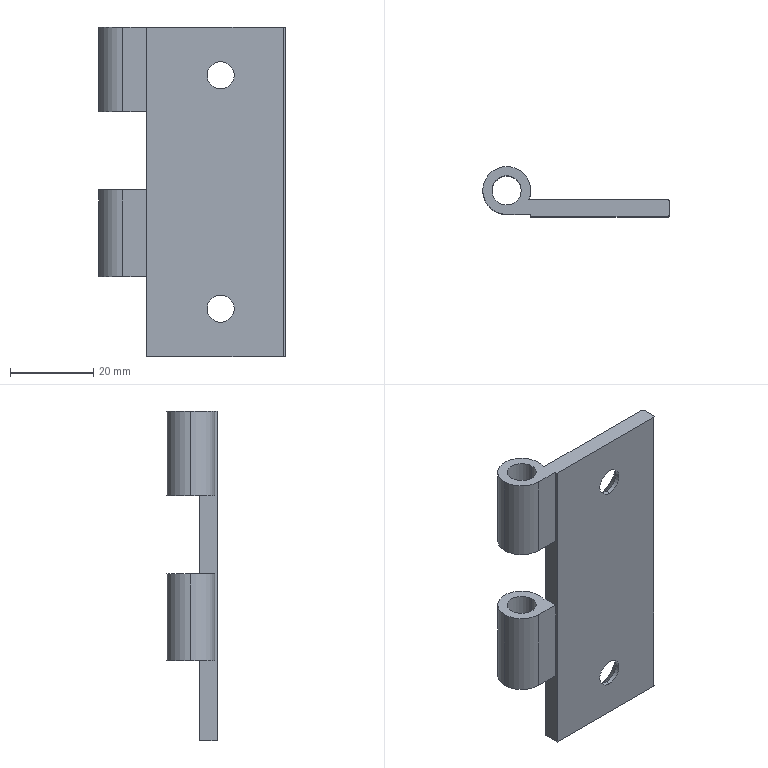Part | SolidWorks | features BaseBody 1 | 1 solid | 31 faces | box 44.75 x 12.05 x 79 mm | volume 13207 mm3 | cylinder 16 | plane 11 | cone 4 | commonest cylinder face diameters 11.5 x6 6.5 x4 7 x4 1 x2
STEP:
#1=CARTESIAN_POINT('',(23.5,0.,-24.75));
#2=VERTEX_POINT('',#1);
#3=CARTESIAN_POINT('',(23.5,0.,-31.25));
#4=VERTEX_POINT('',#3);
#5=CARTESIAN_POINT('',(23.5,0.,-28.));
#6=DIRECTION('',(0.,-1.,0.));
#7=DIRECTION('',(0.,0.,1.));
#8=AXIS2_PLACEMENT_3D('',#5,#6,#7);
#9=CIRCLE('',#8,3.25);
#10=EDGE_CURVE('',#2,#4,#9,.T.);
#11=ORIENTED_EDGE('',*,*,#10,.T.);
#12=CARTESIAN_POINT('',(23.5,1.1,-31.25));
#13=VERTEX_POINT('',#12);
#14=CARTESIAN_POINT('',(23.5,0.,-31.25));
#15=DIRECTION('',(0.,1.,0.));
#16=VECTOR('',#15,1000.);
#17=LINE('',#14,#16);
#18=EDGE_CURVE('',#4,#13,#17,.T.);
#19=ORIENTED_EDGE('',*,*,#18,.T.);
#20=CARTESIAN_POINT('',(23.5,1.1,-24.75));
#21=VERTEX_POINT('',#20);
#22=CARTESIAN_POINT('',(23.5,1.1,-28.));
#23=DIRECTION('',(0.,-1.,0.));
#24=DIRECTION('',(0.,0.,1.));
#25=AXIS2_PLACEMENT_3D('',#22,#23,#24);
#26=CIRCLE('',#25,3.25);
#27=EDGE_CURVE('',#21,#13,#26,.T.);
#28=ORIENTED_EDGE('',*,*,#27,.F.);
#29=CARTESIAN_POINT('',(23.5,0.,-24.75));
#30=DIRECTION('',(0.,1.,0.));
#31=VECTOR('',#30,1000.);
#32=LINE('',#29,#31);
#33=EDGE_CURVE('',#2,#21,#32,.T.);
#34=ORIENTED_EDGE('',*,*,#33,.F.);
#35=EDGE_LOOP('',(#11,#19,#28,#34));
#36=FACE_OUTER_BOUND('',#35,.T.);
#37=CARTESIAN_POINT('',(23.5,0.,-28.));
#38=DIRECTION('',(0.,1.,0.));
#39=DIRECTION('',(0.,0.,1.));
#40=AXIS2_PLACEMENT_3D('',#37,#38,#39);
#41=CYLINDRICAL_SURFACE('',#40,3.25);
#42=ADVANCED_FACE('',(#36),#41,.F.);
#43=CARTESIAN_POINT('',(23.5,0.,31.25));
#44=VERTEX_POINT('',#43);
#45=CARTESIAN_POINT('',(23.5,0.,24.75));
#46=VERTEX_POINT('',#45);
#47=CARTESIAN_POINT('',(23.5,0.,28.));
#48=DIRECTION('',(0.,-1.,0.));
#49=DIRECTION('',(0.,0.,1.));
#50=AXIS2_PLACEMENT_3D('',#47,#48,#49);
#51=CIRCLE('',#50,3.25);
#52=EDGE_CURVE('',#44,#46,#51,.T.);
#53=ORIENTED_EDGE('',*,*,#52,.T.);
#54=CARTESIAN_POINT('',(23.5,1.1,24.75));
#55=VERTEX_POINT('',#54);
#56=CARTESIAN_POINT('',(23.5,0.,24.75));
#57=DIRECTION('',(0.,1.,0.));
#58=VECTOR('',#57,1000.);
#59=LINE('',#56,#58);
#60=EDGE_CURVE('',#46,#55,#59,.T.);
#61=ORIENTED_EDGE('',*,*,#60,.T.);
#62=CARTESIAN_POINT('',(23.5,1.1,31.25));
#63=VERTEX_POINT('',#62);
#64=CARTESIAN_POINT('',(23.5,1.1,28.));
#65=DIRECTION('',(0.,-1.,0.));
#66=DIRECTION('',(0.,0.,1.));
#67=AXIS2_PLACEMENT_3D('',#64,#65,#66);
#68=CIRCLE('',#67,3.25);
#69=EDGE_CURVE('',#63,#55,#68,.T.);
#70=ORIENTED_EDGE('',*,*,#69,.F.);
#71=CARTESIAN_POINT('',(23.5,0.,31.25));
#72=DIRECTION('',(0.,1.,0.));
#73=VECTOR('',#72,1000.);
#74=LINE('',#71,#73);
#75=EDGE_CURVE('',#44,#63,#74,.T.);
#76=ORIENTED_EDGE('',*,*,#75,.F.);
#77=EDGE_LOOP('',(#53,#61,#70,#76));
#78=FACE_OUTER_BOUND('',#77,.T.);
#79=CARTESIAN_POINT('',(23.5,0.,28.));
#80=DIRECTION('',(0.,1.,0.));
#81=DIRECTION('',(0.,0.,1.));
#82=AXIS2_PLACEMENT_3D('',#79,#80,#81);
#83=CYLINDRICAL_SURFACE('',#82,3.25);
#84=ADVANCED_FACE('',(#78),#83,.F.);
#85=CARTESIAN_POINT('',(5.75,6.3,19.3));
#86=VERTEX_POINT('',#85);
#87=CARTESIAN_POINT('',(-5.75,6.3,19.3));
#88=VERTEX_POINT('',#87);
#89=CARTESIAN_POINT('',(0.,6.3,19.3));
#90=DIRECTION('',(0.,0.,1.));
#91=DIRECTION('',(1.,0.,0.));
#92=AXIS2_PLACEMENT_3D('',#89,#90,#91);
#93=CIRCLE('',#92,5.75);
#94=EDGE_CURVE('',#86,#88,#93,.T.);
#95=ORIENTED_EDGE('',*,*,#94,.T.);
#96=CARTESIAN_POINT('',(-5.75,6.3,39.5));
#97=VERTEX_POINT('',#96);
#98=CARTESIAN_POINT('',(-5.75,6.3,39.5));
#99=DIRECTION('',(0.,0.,1.));
#100=VECTOR('',#99,1000.);
#101=LINE('',#98,#100);
#102=EDGE_CURVE('',#88,#97,#101,.T.);
#103=ORIENTED_EDGE('',*,*,#102,.T.);
#104=CARTESIAN_POINT('',(5.75,6.3,39.5));
#105=VERTEX_POINT('',#104);
#106=CARTESIAN_POINT('',(0.,6.3,39.5));
#107=DIRECTION('',(0.,0.,1.));
#108=DIRECTION('',(1.,0.,0.));
#109=AXIS2_PLACEMENT_3D('',#106,#107,#108);
#110=CIRCLE('',#109,5.75);
#111=EDGE_CURVE('',#105,#97,#110,.T.);
#112=ORIENTED_EDGE('',*,*,#111,.F.);
#113=CARTESIAN_POINT('',(5.75,6.3,39.5));
#114=DIRECTION('',(0.,0.,1.));
#115=VECTOR('',#114,1000.);
#116=LINE('',#113,#115);
#117=EDGE_CURVE('',#86,#105,#116,.T.);
#118=ORIENTED_EDGE('',*,*,#117,.F.);
#119=EDGE_LOOP('',(#95,#103,#112,#118));
#120=FACE_OUTER_BOUND('',#119,.T.);
#121=CARTESIAN_POINT('',(0.,6.3,39.5));
#122=DIRECTION('',(0.,0.,1.));
#123=DIRECTION('',(1.,0.,0.));
#124=AXIS2_PLACEMENT_3D('',#121,#122,#123);
#125=CYLINDRICAL_SURFACE('',#124,5.75);
#126=ADVANCED_FACE('',(#120),#125,.T.);
#127=CARTESIAN_POINT('',(5.312,4.1,19.3));
#128=VERTEX_POINT('',#127);
#129=CARTESIAN_POINT('',(0.,6.3,19.3));
#130=DIRECTION('',(0.,0.,1.));
#131=DIRECTION('',(1.,0.,0.));
#132=AXIS2_PLACEMENT_3D('',#129,#130,#131);
#133=CIRCLE('',#132,5.75);
#134=EDGE_CURVE('',#128,#86,#133,.T.);
#135=ORIENTED_EDGE('',*,*,#134,.T.);
#136=ORIENTED_EDGE('',*,*,#117,.T.);
#137=CARTESIAN_POINT('',(5.312,4.1,39.5));
#138=VERTEX_POINT('',#137);
#139=CARTESIAN_POINT('',(0.,6.3,39.5));
#140=DIRECTION('',(0.,0.,1.));
#141=DIRECTION('',(1.,0.,0.));
#142=AXIS2_PLACEMENT_3D('',#139,#140,#141);
#143=CIRCLE('',#142,5.75);
#144=EDGE_CURVE('',#138,#105,#143,.T.);
#145=ORIENTED_EDGE('',*,*,#144,.F.);
#146=CARTESIAN_POINT('',(5.312,4.1,39.5));
#147=DIRECTION('',(0.,0.,-1.));
#148=VECTOR('',#147,1000.);
#149=LINE('',#146,#148);
#150=EDGE_CURVE('',#138,#128,#149,.T.);
#151=ORIENTED_EDGE('',*,*,#150,.T.);
#152=EDGE_LOOP('',(#135,#136,#145,#151));
#153=FACE_OUTER_BOUND('',#152,.T.);
#154=CARTESIAN_POINT('',(0.,6.3,39.5));
#155=DIRECTION('',(0.,0.,1.));
#156=DIRECTION('',(1.,0.,0.));
#157=AXIS2_PLACEMENT_3D('',#154,#155,#156);
#158=CYLINDRICAL_SURFACE('',#157,5.75);
#159=ADVANCED_FACE('',(#153),#158,.T.);
#160=CARTESIAN_POINT('',(-3.5,6.3,19.3));
#161=VERTEX_POINT('',#160);
#162=CARTESIAN_POINT('',(3.5,6.3,19.3));
#163=VERTEX_POINT('',#162);
#164=CARTESIAN_POINT('',(0.,6.3,19.3));
#165=DIRECTION('',(0.,0.,1.));
#166=DIRECTION('',(1.,0.,0.));
#167=AXIS2_PLACEMENT_3D('',#164,#165,#166);
#168=CIRCLE('',#167,3.5);
#169=EDGE_CURVE('',#161,#163,#168,.T.);
#170=ORIENTED_EDGE('',*,*,#169,.F.);
#171=CARTESIAN_POINT('',(-3.5,6.3,39.5));
#172=VERTEX_POINT('',#171);
#173=CARTESIAN_POINT('',(-3.5,6.3,39.5));
#174=DIRECTION('',(0.,0.,1.));
#175=VECTOR('',#174,1000.);
#176=LINE('',#173,#175);
#177=EDGE_CURVE('',#161,#172,#176,.T.);
#178=ORIENTED_EDGE('',*,*,#177,.T.);
#179=CARTESIAN_POINT('',(3.5,6.3,39.5));
#180=VERTEX_POINT('',#179);
#181=CARTESIAN_POINT('',(0.,6.3,39.5));
#182=DIRECTION('',(0.,0.,-1.));
#183=DIRECTION('',(1.,0.,0.));
#184=AXIS2_PLACEMENT_3D('',#181,#182,#183);
#185=CIRCLE('',#184,3.5);
#186=EDGE_CURVE('',#180,#172,#185,.T.);
#187=ORIENTED_EDGE('',*,*,#186,.F.);
#188=CARTESIAN_POINT('',(3.5,6.3,39.5));
#189=DIRECTION('',(0.,0.,1.));
#190=VECTOR('',#189,1000.);
#191=LINE('',#188,#190);
#192=EDGE_CURVE('',#163,#180,#191,.T.);
#193=ORIENTED_EDGE('',*,*,#192,.F.);
#194=EDGE_LOOP('',(#170,#178,#187,#193));
#195=FACE_OUTER_BOUND('',#194,.T.);
#196=CARTESIAN_POINT('',(0.,6.3,39.5));
#197=DIRECTION('',(0.,0.,1.));
#198=DIRECTION('',(1.,0.,0.));
#199=AXIS2_PLACEMENT_3D('',#196,#197,#198);
#200=CYLINDRICAL_SURFACE('',#199,3.5);
#201=ADVANCED_FACE('',(#195),#200,.F.);
#202=ORIENTED_EDGE('',*,*,#27,.T.);
#203=CARTESIAN_POINT('',(23.5,4.1,-34.25));
#204=VERTEX_POINT('',#203);
#205=CARTESIAN_POINT('',(23.5,4.1,-34.25));
#206=DIRECTION('',(0.,0.7071,-0.7071));
#207=VECTOR('',#206,1000.);
#208=LINE('',#205,#207);
#209=EDGE_CURVE('',#13,#204,#208,.T.);
#210=ORIENTED_EDGE('',*,*,#209,.T.);
#211=CARTESIAN_POINT('',(23.5,4.1,-21.75));
#212=VERTEX_POINT('',#211);
#213=CARTESIAN_POINT('',(23.5,4.1,-28.));
#214=DIRECTION('',(0.,1.,0.));
#215=DIRECTION('',(0.,0.,1.));
#216=AXIS2_PLACEMENT_3D('',#213,#214,#215);
#217=CIRCLE('',#216,6.25);
#218=EDGE_CURVE('',#204,#212,#217,.T.);
#219=ORIENTED_EDGE('',*,*,#218,.T.);
#220=CARTESIAN_POINT('',(23.5,4.1,-21.75));
#221=DIRECTION('',(0.,0.7071,0.7071));
#222=VECTOR('',#221,1000.);
#223=LINE('',#220,#222);
#224=EDGE_CURVE('',#21,#212,#223,.T.);
#225=ORIENTED_EDGE('',*,*,#224,.F.);
#226=EDGE_LOOP('',(#202,#210,#219,#225));
#227=FACE_OUTER_BOUND('',#226,.T.);
#228=CARTESIAN_POINT('',(23.5,4.1,-28.));
#229=DIRECTION('',(0.,1.,0.));
#230=DIRECTION('',(0.,0.,1.));
#231=AXIS2_PLACEMENT_3D('',#228,#229,#230);
#232=CONICAL_SURFACE('',#231,6.25,0.7854);
#233=ADVANCED_FACE('',(#227),#232,.F.);
#234=ORIENTED_EDGE('',*,*,#69,.T.);
#235=CARTESIAN_POINT('',(23.5,4.1,21.75));
#236=VERTEX_POINT('',#235);
#237=CARTESIAN_POINT('',(23.5,4.1,21.75));
#238=DIRECTION('',(0.,0.7071,-0.7071));
#239=VECTOR('',#238,1000.);
#240=LINE('',#237,#239);
#241=EDGE_CURVE('',#55,#236,#240,.T.);
#242=ORIENTED_EDGE('',*,*,#241,.T.);
#243=CARTESIAN_POINT('',(23.5,4.1,34.25));
#244=VERTEX_POINT('',#243);
#245=CARTESIAN_POINT('',(23.5,4.1,28.));
#246=DIRECTION('',(0.,1.,0.));
#247=DIRECTION('',(0.,0.,1.));
#248=AXIS2_PLACEMENT_3D('',#245,#246,#247);
#249=CIRCLE('',#248,6.25);
#250=EDGE_CURVE('',#236,#244,#249,.T.);
#251=ORIENTED_EDGE('',*,*,#250,.T.);
#252=CARTESIAN_POINT('',(23.5,4.1,34.25));
#253=DIRECTION('',(0.,0.7071,0.7071));
#254=VECTOR('',#253,1000.);
#255=LINE('',#252,#254);
#256=EDGE_CURVE('',#63,#244,#255,.T.);
#257=ORIENTED_EDGE('',*,*,#256,.F.);
#258=EDGE_LOOP('',(#234,#242,#251,#257));
#259=FACE_OUTER_BOUND('',#258,.T.);
#260=CARTESIAN_POINT('',(23.5,4.1,28.));
#261=DIRECTION('',(0.,1.,0.));
#262=DIRECTION('',(0.,0.,1.));
#263=AXIS2_PLACEMENT_3D('',#260,#261,#262);
#264=CONICAL_SURFACE('',#263,6.25,0.7854);
#265=ADVANCED_FACE('',(#259),#264,.F.);
#266=CARTESIAN_POINT('',(-5.75,6.3,-20.3));
#267=VERTEX_POINT('',#266);
#268=CARTESIAN_POINT('',(5.75,6.3,-20.3));
#269=VERTEX_POINT('',#268);
#270=CARTESIAN_POINT('',(0.,6.3,-20.3));
#271=DIRECTION('',(0.,0.,-1.));
#272=DIRECTION('',(1.,0.,0.));
#273=AXIS2_PLACEMENT_3D('',#270,#271,#272);
#274=CIRCLE('',#273,5.75);
#275=EDGE_CURVE('',#267,#269,#274,.T.);
#276=ORIENTED_EDGE('',*,*,#275,.F.);
#277=CARTESIAN_POINT('',(-5.75,6.3,0.5));
#278=VERTEX_POINT('',#277);
#279=CARTESIAN_POINT('',(-5.75,6.3,39.5));
#280=DIRECTION('',(0.,0.,1.));
#281=VECTOR('',#280,1000.);
#282=LINE('',#279,#281);
#283=EDGE_CURVE('',#267,#278,#282,.T.);
#284=ORIENTED_EDGE('',*,*,#283,.T.);
#285=CARTESIAN_POINT('',(5.75,6.3,0.5));
#286=VERTEX_POINT('',#285);
#287=CARTESIAN_POINT('',(0.,6.3,0.5));
#288=DIRECTION('',(0.,0.,1.));
#289=DIRECTION('',(1.,0.,0.));
#290=AXIS2_PLACEMENT_3D('',#287,#288,#289);
#291=CIRCLE('',#290,5.75);
#292=EDGE_CURVE('',#286,#278,#291,.T.);
#293=ORIENTED_EDGE('',*,*,#292,.F.);
#294=CARTESIAN_POINT('',(5.75,6.3,39.5));
#295=DIRECTION('',(0.,0.,1.));
#296=VECTOR('',#295,1000.);
#297=LINE('',#294,#296);
#298=EDGE_CURVE('',#269,#286,#297,.T.);
#299=ORIENTED_EDGE('',*,*,#298,.F.);
#300=EDGE_LOOP('',(#276,#284,#293,#299));
#301=FACE_OUTER_BOUND('',#300,.T.);
#302=CARTESIAN_POINT('',(0.,6.3,39.5));
#303=DIRECTION('',(0.,0.,1.));
#304=DIRECTION('',(1.,0.,0.));
#305=AXIS2_PLACEMENT_3D('',#302,#303,#304);
#306=CYLINDRICAL_SURFACE('',#305,5.75);
#307=ADVANCED_FACE('',(#301),#306,.T.);
#308=CARTESIAN_POINT('',(5.312,4.1,-20.3));
#309=VERTEX_POINT('',#308);
#310=CARTESIAN_POINT('',(0.,6.3,-20.3));
#311=DIRECTION('',(0.,0.,-1.));
#312=DIRECTION('',(1.,0.,0.));
#313=AXIS2_PLACEMENT_3D('',#310,#311,#312);
#314=CIRCLE('',#313,5.75);
#315=EDGE_CURVE('',#269,#309,#314,.T.);
#316=ORIENTED_EDGE('',*,*,#315,.F.);
#317=ORIENTED_EDGE('',*,*,#298,.T.);
#318=CARTESIAN_POINT('',(5.312,4.1,0.5));
#319=VERTEX_POINT('',#318);
#320=CARTESIAN_POINT('',(0.,6.3,0.5));
#321=DIRECTION('',(0.,0.,1.));
#322=DIRECTION('',(1.,0.,0.));
#323=AXIS2_PLACEMENT_3D('',#320,#321,#322);
#324=CIRCLE('',#323,5.75);
#325=EDGE_CURVE('',#319,#286,#324,.T.);
#326=ORIENTED_EDGE('',*,*,#325,.F.);
#327=CARTESIAN_POINT('',(5.312,4.1,39.5));
#328=DIRECTION('',(0.,0.,-1.));
#329=VECTOR('',#328,1000.);
#330=LINE('',#327,#329);
#331=EDGE_CURVE('',#319,#309,#330,.T.);
#332=ORIENTED_EDGE('',*,*,#331,.T.);
#333=EDGE_LOOP('',(#316,#317,#326,#332));
#334=FACE_OUTER_BOUND('',#333,.T.);
#335=CARTESIAN_POINT('',(0.,6.3,39.5));
#336=DIRECTION('',(0.,0.,1.));
#337=DIRECTION('',(1.,0.,0.));
#338=AXIS2_PLACEMENT_3D('',#335,#336,#337);
#339=CYLINDRICAL_SURFACE('',#338,5.75);
#340=ADVANCED_FACE('',(#334),#339,.T.);
#341=CARTESIAN_POINT('',(-3.5,6.3,-20.3));
#342=VERTEX_POINT('',#341);
#343=CARTESIAN_POINT('',(3.5,6.3,-20.3));
#344=VERTEX_POINT('',#343);
#345=CARTESIAN_POINT('',(0.,6.3,-20.3));
#346=DIRECTION('',(0.,0.,1.));
#347=DIRECTION('',(1.,0.,0.));
#348=AXIS2_PLACEMENT_3D('',#345,#346,#347);
#349=CIRCLE('',#348,3.5);
#350=EDGE_CURVE('',#342,#344,#349,.T.);
#351=ORIENTED_EDGE('',*,*,#350,.F.);
#352=CARTESIAN_POINT('',(-3.5,6.3,0.5));
#353=VERTEX_POINT('',#352);
#354=CARTESIAN_POINT('',(-3.5,6.3,39.5));
#355=DIRECTION('',(0.,0.,1.));
#356=VECTOR('',#355,1000.);
#357=LINE('',#354,#356);
#358=EDGE_CURVE('',#342,#353,#357,.T.);
#359=ORIENTED_EDGE('',*,*,#358,.T.);
#360=CARTESIAN_POINT('',(3.5,6.3,0.5));
#361=VERTEX_POINT('',#360);
#362=CARTESIAN_POINT('',(0.,6.3,0.5));
#363=DIRECTION('',(0.,0.,-1.));
#364=DIRECTION('',(1.,0.,0.));
#365=AXIS2_PLACEMENT_3D('',#362,#363,#364);
#366=CIRCLE('',#365,3.5);
#367=EDGE_CURVE('',#361,#353,#366,.T.);
#368=ORIENTED_EDGE('',*,*,#367,.F.);
#369=CARTESIAN_POINT('',(3.5,6.3,39.5));
#370=DIRECTION('',(0.,0.,1.));
#371=VECTOR('',#370,1000.);
#372=LINE('',#369,#371);
#373=EDGE_CURVE('',#344,#361,#372,.T.);
#374=ORIENTED_EDGE('',*,*,#373,.F.);
#375=EDGE_LOOP('',(#351,#359,#368,#374));
#376=FACE_OUTER_BOUND('',#375,.T.);
#377=CARTESIAN_POINT('',(0.,6.3,39.5));
#378=DIRECTION('',(0.,0.,1.));
#379=DIRECTION('',(1.,0.,0.));
#380=AXIS2_PLACEMENT_3D('',#377,#378,#379);
#381=CYLINDRICAL_SURFACE('',#380,3.5);
#382=ADVANCED_FACE('',(#376),#381,.F.);
#383=CARTESIAN_POINT('',(38.5,0.,39.5));
#384=VERTEX_POINT('',#383);
#385=CARTESIAN_POINT('',(38.5,0.,-39.5));
#386=VERTEX_POINT('',#385);
#387=CARTESIAN_POINT('',(38.5,0.,39.5));
#388=DIRECTION('',(0.,0.,-1.));
#389=VECTOR('',#388,1000.);
#390=LINE('',#387,#389);
#391=EDGE_CURVE('',#384,#386,#390,.T.);
#392=ORIENTED_EDGE('',*,*,#391,.F.);
#393=CARTESIAN_POINT('',(5.75,0.,39.5));
#394=VERTEX_POINT('',#393);
#395=CARTESIAN_POINT('',(5.75,0.,39.5));
#396=DIRECTION('',(1.,0.,0.));
#397=VECTOR('',#396,1000.);
#398=LINE('',#395,#397);
#399=EDGE_CURVE('',#394,#384,#398,.T.);
#400=ORIENTED_EDGE('',*,*,#399,.F.);
#401=CARTESIAN_POINT('',(5.75,0.,-39.5));
#402=VERTEX_POINT('',#401);
#403=CARTESIAN_POINT('',(5.75,0.,39.5));
#404=DIRECTION('',(0.,0.,1.));
#405=VECTOR('',#404,1000.);
#406=LINE('',#403,#405);
#407=EDGE_CURVE('',#402,#394,#406,.T.);
#408=ORIENTED_EDGE('',*,*,#407,.F.);
#409=CARTESIAN_POINT('',(5.75,0.,-39.5));
#410=DIRECTION('',(-1.,0.,0.));
#411=VECTOR('',#410,1000.);
#412=LINE('',#409,#411);
#413=EDGE_CURVE('',#386,#402,#412,.T.);
#414=ORIENTED_EDGE('',*,*,#413,.F.);
#415=EDGE_LOOP('',(#392,#400,#408,#414));
#416=FACE_OUTER_BOUND('',#415,.T.);
#417=ORIENTED_EDGE('',*,*,#10,.F.);
#418=CARTESIAN_POINT('',(23.5,0.,-28.));
#419=DIRECTION('',(0.,-1.,0.));
#420=DIRECTION('',(0.,0.,1.));
#421=AXIS2_PLACEMENT_3D('',#418,#419,#420);
#422=CIRCLE('',#421,3.25);
#423=EDGE_CURVE('',#4,#2,#422,.T.);
#424=ORIENTED_EDGE('',*,*,#423,.F.);
#425=EDGE_LOOP('',(#417,#424));
#426=FACE_BOUND('',#425,.T.);
#427=ORIENTED_EDGE('',*,*,#52,.F.);
#428=CARTESIAN_POINT('',(23.5,0.,28.));
#429=DIRECTION('',(0.,-1.,0.));
#430=DIRECTION('',(0.,0.,1.));
#431=AXIS2_PLACEMENT_3D('',#428,#429,#430);
#432=CIRCLE('',#431,3.25);
#433=EDGE_CURVE('',#46,#44,#432,.T.);
#434=ORIENTED_EDGE('',*,*,#433,.F.);
#435=EDGE_LOOP('',(#427,#434));
#436=FACE_BOUND('',#435,.T.);
#437=CARTESIAN_POINT('',(5.75,0.,39.5));
#438=DIRECTION('',(0.,1.,0.));
#439=DIRECTION('',(0.,0.,1.));
#440=AXIS2_PLACEMENT_3D('',#437,#438,#439);
#441=PLANE('',#440);
#442=ADVANCED_FACE('',(#416,#426,#436),#441,.F.);
#443=CARTESIAN_POINT('',(38.5,4.1,-39.5));
#444=VERTEX_POINT('',#443);
#445=CARTESIAN_POINT('',(5.75,4.1,-39.5));
#446=VERTEX_POINT('',#445);
#447=CARTESIAN_POINT('',(0.,4.1,-39.5));
#448=DIRECTION('',(-1.,0.,0.));
#449=VECTOR('',#448,1000.);
#450=LINE('',#447,#449);
#451=EDGE_CURVE('',#444,#446,#450,.T.);
#452=ORIENTED_EDGE('',*,*,#451,.F.);
#453=CARTESIAN_POINT('',(39.,3.6,-39.5));
#454=VERTEX_POINT('',#453);
#455=CARTESIAN_POINT('',(38.5,3.6,-39.5));
#456=DIRECTION('',(0.,0.,1.));
#457=DIRECTION('',(1.,0.,0.));
#458=AXIS2_PLACEMENT_3D('',#455,#456,#457);
#459=CIRCLE('',#458,0.5);
#460=EDGE_CURVE('',#454,#444,#459,.T.);
#461=ORIENTED_EDGE('',*,*,#460,.F.);
#462=CARTESIAN_POINT('',(39.,0.5,-39.5));
#463=VERTEX_POINT('',#462);
#464=CARTESIAN_POINT('',(39.,6.3,-39.5));
#465=DIRECTION('',(0.,1.,0.));
#466=VECTOR('',#465,1000.);
#467=LINE('',#464,#466);
#468=EDGE_CURVE('',#463,#454,#467,.T.);
#469=ORIENTED_EDGE('',*,*,#468,.F.);
#470=CARTESIAN_POINT('',(38.5,0.5,-39.5));
#471=DIRECTION('',(0.,0.,1.));
#472=DIRECTION('',(1.,0.,0.));
#473=AXIS2_PLACEMENT_3D('',#470,#471,#472);
#474=CIRCLE('',#473,0.5);
#475=EDGE_CURVE('',#386,#463,#474,.T.);
#476=ORIENTED_EDGE('',*,*,#475,.F.);
#477=ORIENTED_EDGE('',*,*,#413,.T.);
#478=CARTESIAN_POINT('',(5.75,6.3,-39.5));
#479=DIRECTION('',(0.,-1.,0.));
#480=VECTOR('',#479,1000.);
#481=LINE('',#478,#480);
#482=EDGE_CURVE('',#446,#402,#481,.T.);
#483=ORIENTED_EDGE('',*,*,#482,.F.);
#484=EDGE_LOOP('',(#452,#461,#469,#476,#477,#483));
#485=FACE_OUTER_BOUND('',#484,.T.);
#486=CARTESIAN_POINT('',(0.,6.3,-39.5));
#487=DIRECTION('',(0.,0.,1.));
#488=DIRECTION('',(1.,0.,0.));
#489=AXIS2_PLACEMENT_3D('',#486,#487,#488);
#490=PLANE('',#489);
#491=ADVANCED_FACE('',(#485),#490,.F.);
#492=CARTESIAN_POINT('',(39.,0.5,39.5));
#493=VERTEX_POINT('',#492);
#494=CARTESIAN_POINT('',(38.5,0.5,39.5));
#495=DIRECTION('',(0.,0.,-1.));
#496=DIRECTION('',(1.,0.,0.));
#497=AXIS2_PLACEMENT_3D('',#494,#495,#496);
#498=CIRCLE('',#497,0.5);
#499=EDGE_CURVE('',#493,#384,#498,.T.);
#500=ORIENTED_EDGE('',*,*,#499,.T.);
#501=ORIENTED_EDGE('',*,*,#391,.T.);
#502=ORIENTED_EDGE('',*,*,#475,.T.);
#503=CARTESIAN_POINT('',(39.,0.5,39.5));
#504=DIRECTION('',(0.,0.,1.));
#505=VECTOR('',#504,1000.);
#506=LINE('',#503,#505);
#507=EDGE_CURVE('',#463,#493,#506,.T.);
#508=ORIENTED_EDGE('',*,*,#507,.T.);
#509=EDGE_LOOP('',(#500,#501,#502,#508));
#510=FACE_OUTER_BOUND('',#509,.T.);
#511=CARTESIAN_POINT('',(38.5,0.5,39.5));
#512=DIRECTION('',(0.,0.,1.));
#513=DIRECTION('',(1.,0.,0.));
#514=AXIS2_PLACEMENT_3D('',#511,#512,#513);
#515=CYLINDRICAL_SURFACE('',#514,0.5);
#516=ADVANCED_FACE('',(#510),#515,.T.);
#517=CARTESIAN_POINT('',(39.,3.6,39.5));
#518=VERTEX_POINT('',#517);
#519=CARTESIAN_POINT('',(39.,6.3,39.5));
#520=DIRECTION('',(0.,1.,0.));
#521=VECTOR('',#520,1000.);
#522=LINE('',#519,#521);
#523=EDGE_CURVE('',#493,#518,#522,.T.);
#524=ORIENTED_EDGE('',*,*,#523,.T.);
#525=CARTESIAN_POINT('',(38.5,4.1,39.5));
#526=VERTEX_POINT('',#525);
#527=CARTESIAN_POINT('',(38.5,3.6,39.5));
#528=DIRECTION('',(0.,0.,-1.));
#529=DIRECTION('',(1.,0.,0.));
#530=AXIS2_PLACEMENT_3D('',#527,#528,#529);
#531=CIRCLE('',#530,0.5);
#532=EDGE_CURVE('',#526,#518,#531,.T.);
#533=ORIENTED_EDGE('',*,*,#532,.F.);
#534=CARTESIAN_POINT('',(0.,4.1,39.5));
#535=DIRECTION('',(-1.,0.,0.));
#536=VECTOR('',#535,1000.);
#537=LINE('',#534,#536);
#538=EDGE_CURVE('',#526,#138,#537,.T.);
#539=ORIENTED_EDGE('',*,*,#538,.T.);
#540=ORIENTED_EDGE('',*,*,#144,.T.);
#541=ORIENTED_EDGE('',*,*,#111,.T.);
#542=CARTESIAN_POINT('',(0.,0.55,39.5));
#543=VERTEX_POINT('',#542);
#544=CARTESIAN_POINT('',(0.,6.3,39.5));
#545=DIRECTION('',(0.,0.,1.));
#546=DIRECTION('',(1.,0.,0.));
#547=AXIS2_PLACEMENT_3D('',#544,#545,#546);
#548=CIRCLE('',#547,5.75);
#549=EDGE_CURVE('',#97,#543,#548,.T.);
#550=ORIENTED_EDGE('',*,*,#549,.T.);
#551=CARTESIAN_POINT('',(5.75,0.55,39.5));
#552=VERTEX_POINT('',#551);
#553=CARTESIAN_POINT('',(0.,0.55,39.5));
#554=DIRECTION('',(1.,0.,0.));
#555=VECTOR('',#554,1000.);
#556=LINE('',#553,#555);
#557=EDGE_CURVE('',#543,#552,#556,.T.);
#558=ORIENTED_EDGE('',*,*,#557,.T.);
#559=CARTESIAN_POINT('',(5.75,6.3,39.5));
#560=DIRECTION('',(0.,-1.,0.));
#561=VECTOR('',#560,1000.);
#562=LINE('',#559,#561);
#563=EDGE_CURVE('',#552,#394,#562,.T.);
#564=ORIENTED_EDGE('',*,*,#563,.T.);
#565=ORIENTED_EDGE('',*,*,#399,.T.);
#566=ORIENTED_EDGE('',*,*,#499,.F.);
#567=EDGE_LOOP('',(#524,#533,#539,#540,#541,#550,#558,#564,#565,#566));
#568=FACE_OUTER_BOUND('',#567,.T.);
#569=ORIENTED_EDGE('',*,*,#186,.T.);
#570=CARTESIAN_POINT('',(0.,6.3,39.5));
#571=DIRECTION('',(0.,0.,-1.));
#572=DIRECTION('',(1.,0.,0.));
#573=AXIS2_PLACEMENT_3D('',#570,#571,#572);
#574=CIRCLE('',#573,3.5);
#575=EDGE_CURVE('',#172,#180,#574,.T.);
#576=ORIENTED_EDGE('',*,*,#575,.T.);
#577=EDGE_LOOP('',(#569,#576));
#578=FACE_BOUND('',#577,.T.);
#579=CARTESIAN_POINT('',(0.,6.3,39.5));
#580=DIRECTION('',(0.,0.,1.));
#581=DIRECTION('',(1.,0.,0.));
#582=AXIS2_PLACEMENT_3D('',#579,#580,#581);
#583=PLANE('',#582);
#584=ADVANCED_FACE('',(#568,#578),#583,.T.);
#585=ORIENTED_EDGE('',*,*,#407,.T.);
#586=ORIENTED_EDGE('',*,*,#563,.F.);
#587=CARTESIAN_POINT('',(5.75,0.55,19.3));
#588=VERTEX_POINT('',#587);
#589=CARTESIAN_POINT('',(5.75,0.55,39.5));
#590=DIRECTION('',(0.,0.,1.));
#591=VECTOR('',#590,1000.);
#592=LINE('',#589,#591);
#593=EDGE_CURVE('',#588,#552,#592,.T.);
#594=ORIENTED_EDGE('',*,*,#593,.F.);
#595=CARTESIAN_POINT('',(5.75,4.1,19.3));
#596=VERTEX_POINT('',#595);
#597=CARTESIAN_POINT('',(5.75,0.55,19.3));
#598=DIRECTION('',(0.,-1.,0.));
#599=VECTOR('',#598,1000.);
#600=LINE('',#597,#599);
#601=EDGE_CURVE('',#596,#588,#600,.T.);
#602=ORIENTED_EDGE('',*,*,#601,.F.);
#603=CARTESIAN_POINT('',(5.75,4.1,0.5));
#604=VERTEX_POINT('',#603);
#605=CARTESIAN_POINT('',(5.75,4.1,39.5));
#606=DIRECTION('',(0.,0.,1.));
#607=VECTOR('',#606,1000.);
#608=LINE('',#605,#607);
#609=EDGE_CURVE('',#604,#596,#608,.T.);
#610=ORIENTED_EDGE('',*,*,#609,.F.);
#611=CARTESIAN_POINT('',(5.75,0.55,0.5));
#612=VERTEX_POINT('',#611);
#613=CARTESIAN_POINT('',(5.75,0.55,0.5));
#614=DIRECTION('',(0.,1.,0.));
#615=VECTOR('',#614,1000.);
#616=LINE('',#613,#615);
#617=EDGE_CURVE('',#612,#604,#616,.T.);
#618=ORIENTED_EDGE('',*,*,#617,.F.);
#619=CARTESIAN_POINT('',(5.75,0.55,-20.3));
#620=VERTEX_POINT('',#619);
#621=CARTESIAN_POINT('',(5.75,0.55,39.5));
#622=DIRECTION('',(0.,0.,1.));
#623=VECTOR('',#622,1000.);
#624=LINE('',#621,#623);
#625=EDGE_CURVE('',#620,#612,#624,.T.);
#626=ORIENTED_EDGE('',*,*,#625,.F.);
#627=CARTESIAN_POINT('',(5.75,4.1,-20.3));
#628=VERTEX_POINT('',#627);
#629=CARTESIAN_POINT('',(5.75,0.55,-20.3));
#630=DIRECTION('',(0.,-1.,0.));
#631=VECTOR('',#630,1000.);
#632=LINE('',#629,#631);
#633=EDGE_CURVE('',#628,#620,#632,.T.);
#634=ORIENTED_EDGE('',*,*,#633,.F.);
#635=CARTESIAN_POINT('',(5.75,4.1,39.5));
#636=DIRECTION('',(0.,0.,1.));
#637=VECTOR('',#636,1000.);
#638=LINE('',#635,#637);
#639=EDGE_CURVE('',#446,#628,#638,.T.);
#640=ORIENTED_EDGE('',*,*,#639,.F.);
#641=ORIENTED_EDGE('',*,*,#482,.T.);
#642=EDGE_LOOP('',(#585,#586,#594,#602,#610,#618,#626,#634,#640,#641));
#643=FACE_OUTER_BOUND('',#642,.T.);
#644=CARTESIAN_POINT('',(5.75,0.55,39.5));
#645=DIRECTION('',(1.,0.,0.));
#646=DIRECTION('',(0.,0.,-1.));
#647=AXIS2_PLACEMENT_3D('',#644,#645,#646);
#648=PLANE('',#647);
#649=ADVANCED_FACE('',(#643),#648,.F.);
#650=ORIENTED_EDGE('',*,*,#18,.F.);
#651=ORIENTED_EDGE('',*,*,#423,.T.);
#652=ORIENTED_EDGE('',*,*,#33,.T.);
#653=CARTESIAN_POINT('',(23.5,1.1,-28.));
#654=DIRECTION('',(0.,-1.,0.));
#655=DIRECTION('',(0.,0.,1.));
#656=AXIS2_PLACEMENT_3D('',#653,#654,#655);
#657=CIRCLE('',#656,3.25);
#658=EDGE_CURVE('',#13,#21,#657,.T.);
#659=ORIENTED_EDGE('',*,*,#658,.F.);
#660=EDGE_LOOP('',(#650,#651,#652,#659));
#661=FACE_OUTER_BOUND('',#660,.T.);
#662=CARTESIAN_POINT('',(23.5,0.,-28.));
#663=DIRECTION('',(0.,1.,0.));
#664=DIRECTION('',(0.,0.,1.));
#665=AXIS2_PLACEMENT_3D('',#662,#663,#664);
#666=CYLINDRICAL_SURFACE('',#665,3.25);
#667=ADVANCED_FACE('',(#661),#666,.F.);
#668=ORIENTED_EDGE('',*,*,#60,.F.);
#669=ORIENTED_EDGE('',*,*,#433,.T.);
#670=ORIENTED_EDGE('',*,*,#75,.T.);
#671=CARTESIAN_POINT('',(23.5,1.1,28.));
#672=DIRECTION('',(0.,-1.,0.));
#673=DIRECTION('',(0.,0.,1.));
#674=AXIS2_PLACEMENT_3D('',#671,#672,#673);
#675=CIRCLE('',#674,3.25);
#676=EDGE_CURVE('',#55,#63,#675,.T.);
#677=ORIENTED_EDGE('',*,*,#676,.F.);
#678=EDGE_LOOP('',(#668,#669,#670,#677));
#679=FACE_OUTER_BOUND('',#678,.T.);
#680=CARTESIAN_POINT('',(23.5,0.,28.));
#681=DIRECTION('',(0.,1.,0.));
#682=DIRECTION('',(0.,0.,1.));
#683=AXIS2_PLACEMENT_3D('',#680,#681,#682);
#684=CYLINDRICAL_SURFACE('',#683,3.25);
#685=ADVANCED_FACE('',(#679),#684,.F.);
#686=ORIENTED_EDGE('',*,*,#150,.F.);
#687=ORIENTED_EDGE('',*,*,#538,.F.);
#688=CARTESIAN_POINT('',(38.5,4.1,39.5));
#689=DIRECTION('',(0.,0.,1.));
#690=VECTOR('',#689,1000.);
#691=LINE('',#688,#690);
#692=EDGE_CURVE('',#444,#526,#691,.T.);
#693=ORIENTED_EDGE('',*,*,#692,.F.);
#694=ORIENTED_EDGE('',*,*,#451,.T.);
#695=ORIENTED_EDGE('',*,*,#639,.T.);
#696=CARTESIAN_POINT('',(38.5,4.1,-20.3));
#697=DIRECTION('',(1.,0.,0.));
#698=VECTOR('',#697,1000.);
#699=LINE('',#696,#698);
#700=EDGE_CURVE('',#309,#628,#699,.T.);
#701=ORIENTED_EDGE('',*,*,#700,.F.);
#702=ORIENTED_EDGE('',*,*,#331,.F.);
#703=CARTESIAN_POINT('',(38.5,4.1,0.5));
#704=DIRECTION('',(-1.,0.,0.));
#705=VECTOR('',#704,1000.);
#706=LINE('',#703,#705);
#707=EDGE_CURVE('',#604,#319,#706,.T.);
#708=ORIENTED_EDGE('',*,*,#707,.F.);
#709=ORIENTED_EDGE('',*,*,#609,.T.);
#710=CARTESIAN_POINT('',(38.5,4.1,19.3));
#711=DIRECTION('',(1.,0.,0.));
#712=VECTOR('',#711,1000.);
#713=LINE('',#710,#712);
#714=EDGE_CURVE('',#128,#596,#713,.T.);
#715=ORIENTED_EDGE('',*,*,#714,.F.);
#716=EDGE_LOOP('',(#686,#687,#693,#694,#695,#701,#702,#708,#709,#715));
#717=FACE_OUTER_BOUND('',#716,.T.);
#718=CARTESIAN_POINT('',(23.5,4.1,-28.));
#719=DIRECTION('',(0.,1.,0.));
#720=DIRECTION('',(0.,0.,1.));
#721=AXIS2_PLACEMENT_3D('',#718,#719,#720);
#722=CIRCLE('',#721,6.25);
#723=EDGE_CURVE('',#212,#204,#722,.T.);
#724=ORIENTED_EDGE('',*,*,#723,.F.);
#725=ORIENTED_EDGE('',*,*,#218,.F.);
#726=EDGE_LOOP('',(#724,#725));
#727=FACE_BOUND('',#726,.T.);
#728=CARTESIAN_POINT('',(23.5,4.1,28.));
#729=DIRECTION('',(0.,1.,0.));
#730=DIRECTION('',(0.,0.,1.));
#731=AXIS2_PLACEMENT_3D('',#728,#729,#730);
#732=CIRCLE('',#731,6.25);
#733=EDGE_CURVE('',#244,#236,#732,.T.);
#734=ORIENTED_EDGE('',*,*,#733,.F.);
#735=ORIENTED_EDGE('',*,*,#250,.F.);
#736=EDGE_LOOP('',(#734,#735));
#737=FACE_BOUND('',#736,.T.);
#738=CARTESIAN_POINT('',(38.5,4.1,39.5));
#739=DIRECTION('',(0.,-1.,0.));
#740=DIRECTION('',(0.,0.,-1.));
#741=AXIS2_PLACEMENT_3D('',#738,#739,#740);
#742=PLANE('',#741);
#743=ADVANCED_FACE('',(#717,#727,#737),#742,.F.);
#744=CARTESIAN_POINT('',(39.,3.6,39.5));
#745=DIRECTION('',(0.,0.,-1.));
#746=VECTOR('',#745,1000.);
#747=LINE('',#744,#746);
#748=EDGE_CURVE('',#518,#454,#747,.T.);
#749=ORIENTED_EDGE('',*,*,#748,.F.);
#750=ORIENTED_EDGE('',*,*,#523,.F.);
#751=ORIENTED_EDGE('',*,*,#507,.F.);
#752=ORIENTED_EDGE('',*,*,#468,.T.);
#753=EDGE_LOOP('',(#749,#750,#751,#752));
#754=FACE_OUTER_BOUND('',#753,.T.);
#755=CARTESIAN_POINT('',(39.,0.5,39.5));
#756=DIRECTION('',(-1.,0.,0.));
#757=DIRECTION('',(0.,0.,1.));
#758=AXIS2_PLACEMENT_3D('',#755,#756,#757);
#759=PLANE('',#758);
#760=ADVANCED_FACE('',(#754),#759,.F.);
#761=ORIENTED_EDGE('',*,*,#593,.T.);
#762=ORIENTED_EDGE('',*,*,#557,.F.);
#763=CARTESIAN_POINT('',(0.,0.55,19.3));
#764=VERTEX_POINT('',#763);
#765=CARTESIAN_POINT('',(0.,0.55,39.5));
#766=DIRECTION('',(0.,0.,1.));
#767=VECTOR('',#766,1000.);
#768=LINE('',#765,#767);
#769=EDGE_CURVE('',#764,#543,#768,.T.);
#770=ORIENTED_EDGE('',*,*,#769,.F.);
#771=CARTESIAN_POINT('',(0.,0.55,19.3));
#772=DIRECTION('',(-1.,0.,0.));
#773=VECTOR('',#772,1000.);
#774=LINE('',#771,#773);
#775=EDGE_CURVE('',#588,#764,#774,.T.);
#776=ORIENTED_EDGE('',*,*,#775,.F.);
#777=EDGE_LOOP('',(#761,#762,#770,#776));
#778=FACE_OUTER_BOUND('',#777,.T.);
#779=CARTESIAN_POINT('',(0.,0.55,39.5));
#780=DIRECTION('',(0.,1.,0.));
#781=DIRECTION('',(-1.,0.,0.));
#782=AXIS2_PLACEMENT_3D('',#779,#780,#781);
#783=PLANE('',#782);
#784=ADVANCED_FACE('',(#778),#783,.F.);
#785=ORIENTED_EDGE('',*,*,#102,.F.);
#786=CARTESIAN_POINT('',(0.,6.3,19.3));
#787=DIRECTION('',(0.,0.,1.));
#788=DIRECTION('',(1.,0.,0.));
#789=AXIS2_PLACEMENT_3D('',#786,#787,#788);
#790=CIRCLE('',#789,5.75);
#791=EDGE_CURVE('',#88,#764,#790,.T.);
#792=ORIENTED_EDGE('',*,*,#791,.T.);
#793=ORIENTED_EDGE('',*,*,#769,.T.);
#794=ORIENTED_EDGE('',*,*,#549,.F.);
#795=EDGE_LOOP('',(#785,#792,#793,#794));
#796=FACE_OUTER_BOUND('',#795,.T.);
#797=CARTESIAN_POINT('',(0.,6.3,39.5));
#798=DIRECTION('',(0.,0.,1.));
#799=DIRECTION('',(1.,0.,0.));
#800=AXIS2_PLACEMENT_3D('',#797,#798,#799);
#801=CYLINDRICAL_SURFACE('',#800,5.75);
#802=ADVANCED_FACE('',(#796),#801,.T.);
#803=ORIENTED_EDGE('',*,*,#177,.F.);
#804=CARTESIAN_POINT('',(0.,6.3,19.3));
#805=DIRECTION('',(0.,0.,1.));
#806=DIRECTION('',(1.,0.,0.));
#807=AXIS2_PLACEMENT_3D('',#804,#805,#806);
#808=CIRCLE('',#807,3.5);
#809=EDGE_CURVE('',#163,#161,#808,.T.);
#810=ORIENTED_EDGE('',*,*,#809,.F.);
#811=ORIENTED_EDGE('',*,*,#192,.T.);
#812=ORIENTED_EDGE('',*,*,#575,.F.);
#813=EDGE_LOOP('',(#803,#810,#811,#812));
#814=FACE_OUTER_BOUND('',#813,.T.);
#815=CARTESIAN_POINT('',(0.,6.3,39.5));
#816=DIRECTION('',(0.,0.,1.));
#817=DIRECTION('',(1.,0.,0.));
#818=AXIS2_PLACEMENT_3D('',#815,#816,#817);
#819=CYLINDRICAL_SURFACE('',#818,3.5);
#820=ADVANCED_FACE('',(#814),#819,.F.);
#821=ORIENTED_EDGE('',*,*,#775,.T.);
#822=ORIENTED_EDGE('',*,*,#791,.F.);
#823=ORIENTED_EDGE('',*,*,#94,.F.);
#824=ORIENTED_EDGE('',*,*,#134,.F.);
#825=ORIENTED_EDGE('',*,*,#714,.T.);
#826=ORIENTED_EDGE('',*,*,#601,.T.);
#827=EDGE_LOOP('',(#821,#822,#823,#824,#825,#826));
#828=FACE_OUTER_BOUND('',#827,.T.);
#829=ORIENTED_EDGE('',*,*,#809,.T.);
#830=ORIENTED_EDGE('',*,*,#169,.T.);
#831=EDGE_LOOP('',(#829,#830));
#832=FACE_BOUND('',#831,.T.);
#833=CARTESIAN_POINT('',(-17.25,20.,19.3));
#834=DIRECTION('',(0.,0.,-1.));
#835=DIRECTION('',(-1.,0.,0.));
#836=AXIS2_PLACEMENT_3D('',#833,#834,#835);
#837=PLANE('',#836);
#838=ADVANCED_FACE('',(#828,#832),#837,.T.);
#839=CARTESIAN_POINT('',(0.,0.55,0.5));
#840=VERTEX_POINT('',#839);
#841=CARTESIAN_POINT('',(5.75,0.55,0.5));
#842=DIRECTION('',(1.,0.,0.));
#843=VECTOR('',#842,1000.);
#844=LINE('',#841,#843);
#845=EDGE_CURVE('',#840,#612,#844,.T.);
#846=ORIENTED_EDGE('',*,*,#845,.T.);
#847=ORIENTED_EDGE('',*,*,#617,.T.);
#848=ORIENTED_EDGE('',*,*,#707,.T.);
#849=ORIENTED_EDGE('',*,*,#325,.T.);
#850=ORIENTED_EDGE('',*,*,#292,.T.);
#851=CARTESIAN_POINT('',(0.,6.3,0.5));
#852=DIRECTION('',(0.,0.,1.));
#853=DIRECTION('',(1.,0.,0.));
#854=AXIS2_PLACEMENT_3D('',#851,#852,#853);
#855=CIRCLE('',#854,5.75);
#856=EDGE_CURVE('',#278,#840,#855,.T.);
#857=ORIENTED_EDGE('',*,*,#856,.T.);
#858=EDGE_LOOP('',(#846,#847,#848,#849,#850,#857));
#859=FACE_OUTER_BOUND('',#858,.T.);
#860=ORIENTED_EDGE('',*,*,#367,.T.);
#861=CARTESIAN_POINT('',(0.,6.3,0.5));
#862=DIRECTION('',(0.,0.,-1.));
#863=DIRECTION('',(1.,0.,0.));
#864=AXIS2_PLACEMENT_3D('',#861,#862,#863);
#865=CIRCLE('',#864,3.5);
#866=EDGE_CURVE('',#353,#361,#865,.T.);
#867=ORIENTED_EDGE('',*,*,#866,.T.);
#868=EDGE_LOOP('',(#860,#867));
#869=FACE_BOUND('',#868,.T.);
#870=CARTESIAN_POINT('',(5.75,20.,0.5));
#871=DIRECTION('',(0.,0.,1.));
#872=DIRECTION('',(1.,0.,0.));
#873=AXIS2_PLACEMENT_3D('',#870,#871,#872);
#874=PLANE('',#873);
#875=ADVANCED_FACE('',(#859,#869),#874,.T.);
#876=CARTESIAN_POINT('',(0.,0.55,-20.3));
#877=VERTEX_POINT('',#876);
#878=CARTESIAN_POINT('',(0.,0.55,39.5));
#879=DIRECTION('',(0.,0.,1.));
#880=VECTOR('',#879,1000.);
#881=LINE('',#878,#880);
#882=EDGE_CURVE('',#877,#840,#881,.T.);
#883=ORIENTED_EDGE('',*,*,#882,.F.);
#884=CARTESIAN_POINT('',(0.,0.55,-20.3));
#885=DIRECTION('',(-1.,0.,0.));
#886=VECTOR('',#885,1000.);
#887=LINE('',#884,#886);
#888=EDGE_CURVE('',#620,#877,#887,.T.);
#889=ORIENTED_EDGE('',*,*,#888,.F.);
#890=ORIENTED_EDGE('',*,*,#625,.T.);
#891=ORIENTED_EDGE('',*,*,#845,.F.);
#892=EDGE_LOOP('',(#883,#889,#890,#891));
#893=FACE_OUTER_BOUND('',#892,.T.);
#894=CARTESIAN_POINT('',(0.,0.55,39.5));
#895=DIRECTION('',(0.,1.,0.));
#896=DIRECTION('',(-1.,0.,0.));
#897=AXIS2_PLACEMENT_3D('',#894,#895,#896);
#898=PLANE('',#897);
#899=ADVANCED_FACE('',(#893),#898,.F.);
#900=ORIENTED_EDGE('',*,*,#888,.T.);
#901=CARTESIAN_POINT('',(0.,6.3,-20.3));
#902=DIRECTION('',(0.,0.,-1.));
#903=DIRECTION('',(1.,0.,0.));
#904=AXIS2_PLACEMENT_3D('',#901,#902,#903);
#905=CIRCLE('',#904,5.75);
#906=EDGE_CURVE('',#877,#267,#905,.T.);
#907=ORIENTED_EDGE('',*,*,#906,.T.);
#908=ORIENTED_EDGE('',*,*,#275,.T.);
#909=ORIENTED_EDGE('',*,*,#315,.T.);
#910=ORIENTED_EDGE('',*,*,#700,.T.);
#911=ORIENTED_EDGE('',*,*,#633,.T.);
#912=EDGE_LOOP('',(#900,#907,#908,#909,#910,#911));
#913=FACE_OUTER_BOUND('',#912,.T.);
#914=CARTESIAN_POINT('',(0.,6.3,-20.3));
#915=DIRECTION('',(0.,0.,1.));
#916=DIRECTION('',(1.,0.,0.));
#917=AXIS2_PLACEMENT_3D('',#914,#915,#916);
#918=CIRCLE('',#917,3.5);
#919=EDGE_CURVE('',#344,#342,#918,.T.);
#920=ORIENTED_EDGE('',*,*,#919,.T.);
#921=ORIENTED_EDGE('',*,*,#350,.T.);
#922=EDGE_LOOP('',(#920,#921));
#923=FACE_BOUND('',#922,.T.);
#924=CARTESIAN_POINT('',(-5.75,20.,-20.3));
#925=DIRECTION('',(0.,0.,-1.));
#926=DIRECTION('',(-1.,0.,0.));
#927=AXIS2_PLACEMENT_3D('',#924,#925,#926);
#928=PLANE('',#927);
#929=ADVANCED_FACE('',(#913,#923),#928,.T.);
#930=ORIENTED_EDGE('',*,*,#209,.F.);
#931=ORIENTED_EDGE('',*,*,#658,.T.);
#932=ORIENTED_EDGE('',*,*,#224,.T.);
#933=ORIENTED_EDGE('',*,*,#723,.T.);
#934=EDGE_LOOP('',(#930,#931,#932,#933));
#935=FACE_OUTER_BOUND('',#934,.T.);
#936=CARTESIAN_POINT('',(23.5,4.1,-28.));
#937=DIRECTION('',(0.,1.,0.));
#938=DIRECTION('',(0.,0.,1.));
#939=AXIS2_PLACEMENT_3D('',#936,#937,#938);
#940=CONICAL_SURFACE('',#939,6.25,0.7854);
#941=ADVANCED_FACE('',(#935),#940,.F.);
#942=ORIENTED_EDGE('',*,*,#241,.F.);
#943=ORIENTED_EDGE('',*,*,#676,.T.);
#944=ORIENTED_EDGE('',*,*,#256,.T.);
#945=ORIENTED_EDGE('',*,*,#733,.T.);
#946=EDGE_LOOP('',(#942,#943,#944,#945));
#947=FACE_OUTER_BOUND('',#946,.T.);
#948=CARTESIAN_POINT('',(23.5,4.1,28.));
#949=DIRECTION('',(0.,1.,0.));
#950=DIRECTION('',(0.,0.,1.));
#951=AXIS2_PLACEMENT_3D('',#948,#949,#950);
#952=CONICAL_SURFACE('',#951,6.25,0.7854);
#953=ADVANCED_FACE('',(#947),#952,.F.);
#954=ORIENTED_EDGE('',*,*,#532,.T.);
#955=ORIENTED_EDGE('',*,*,#748,.T.);
#956=ORIENTED_EDGE('',*,*,#460,.T.);
#957=ORIENTED_EDGE('',*,*,#692,.T.);
#958=EDGE_LOOP('',(#954,#955,#956,#957));
#959=FACE_OUTER_BOUND('',#958,.T.);
#960=CARTESIAN_POINT('',(38.5,3.6,39.5));
#961=DIRECTION('',(0.,0.,1.));
#962=DIRECTION('',(1.,0.,0.));
#963=AXIS2_PLACEMENT_3D('',#960,#961,#962);
#964=CYLINDRICAL_SURFACE('',#963,0.5);
#965=ADVANCED_FACE('',(#959),#964,.T.);
#966=ORIENTED_EDGE('',*,*,#283,.F.);
#967=ORIENTED_EDGE('',*,*,#906,.F.);
#968=ORIENTED_EDGE('',*,*,#882,.T.);
#969=ORIENTED_EDGE('',*,*,#856,.F.);
#970=EDGE_LOOP('',(#966,#967,#968,#969));
#971=FACE_OUTER_BOUND('',#970,.T.);
#972=CARTESIAN_POINT('',(0.,6.3,39.5));
#973=DIRECTION('',(0.,0.,1.));
#974=DIRECTION('',(1.,0.,0.));
#975=AXIS2_PLACEMENT_3D('',#972,#973,#974);
#976=CYLINDRICAL_SURFACE('',#975,5.75);
#977=ADVANCED_FACE('',(#971),#976,.T.);
#978=ORIENTED_EDGE('',*,*,#358,.F.);
#979=ORIENTED_EDGE('',*,*,#919,.F.);
#980=ORIENTED_EDGE('',*,*,#373,.T.);
#981=ORIENTED_EDGE('',*,*,#866,.F.);
#982=EDGE_LOOP('',(#978,#979,#980,#981));
#983=FACE_OUTER_BOUND('',#982,.T.);
#984=CARTESIAN_POINT('',(0.,6.3,39.5));
#985=DIRECTION('',(0.,0.,1.));
#986=DIRECTION('',(1.,0.,0.));
#987=AXIS2_PLACEMENT_3D('',#984,#985,#986);
#988=CYLINDRICAL_SURFACE('',#987,3.5);
#989=ADVANCED_FACE('',(#983),#988,.F.);
#990=CLOSED_SHELL('',(#42,#84,#126,#159,#201,#233,#265,#307,#340,#382,#442,#491,#516,#584,#649,#667,#685,#743,#760,#784,#802,#820,#838,#875,#899,#929,#941,#953,#965,#977,#989));
#991=MANIFOLD_SOLID_BREP('',#990);
#992=CARTESIAN_POINT('',(0.,0.,0.));
#993=DIRECTION('',(0.,0.,1.));
#994=DIRECTION('',(1.,0.,0.));
#995=AXIS2_PLACEMENT_3D('',#992,#993,#994);
#996=(LENGTH_UNIT()NAMED_UNIT(*)SI_UNIT(.MILLI.,.METRE.));
#997=UNCERTAINTY_MEASURE_WITH_UNIT(LENGTH_MEASURE(0.00001),#996,'','');
#998=(NAMED_UNIT(*)PLANE_ANGLE_UNIT()SI_UNIT($,.RADIAN.));
#999=(NAMED_UNIT(*)SI_UNIT($,.STERADIAN.)SOLID_ANGLE_UNIT());
#1000=(GEOMETRIC_REPRESENTATION_CONTEXT(3)GLOBAL_UNCERTAINTY_ASSIGNED_CONTEXT((#997))GLOBAL_UNIT_ASSIGNED_CONTEXT((#996,#998,#999))REPRESENTATION_CONTEXT('',''));
#1001=ADVANCED_BREP_SHAPE_REPRESENTATION('',(#991,#995),#1000);